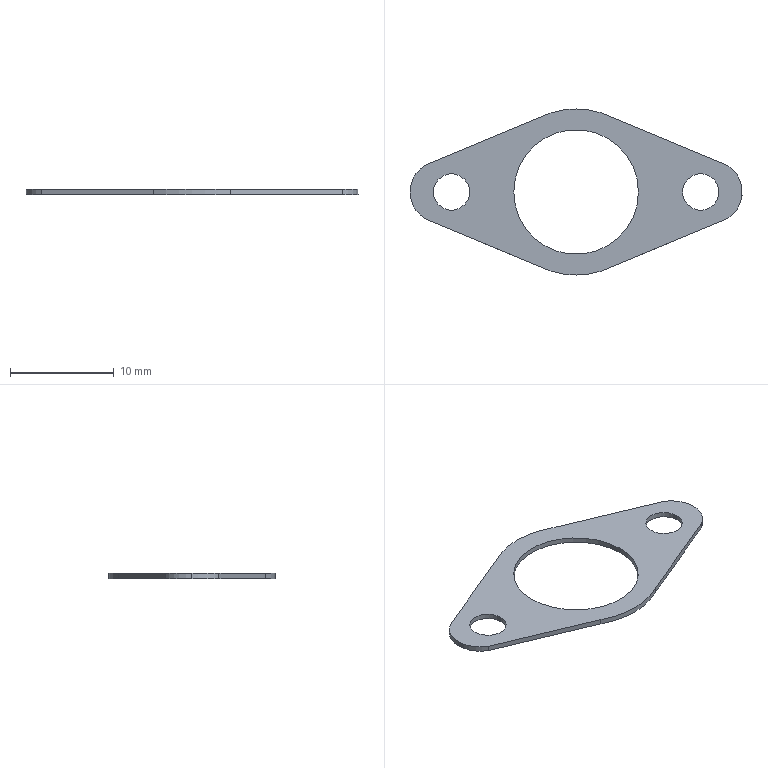Part | STEP file | WENKONG2_1_1_1_1 | 1 solid | 17 faces | box 32 x 16 x 0.5 mm | volume 101.047 mm3 | cylinder 11 | plane 6 | commonest cylinder face diameters 3.5 x4 6 x3 12 x2 16 x2
STEP:
#1=CARTESIAN_POINT('',(0.,0.,0.));
#2=DIRECTION('',(0.,0.,1.));
#3=DIRECTION('',(1.,0.,0.));
#4=AXIS2_PLACEMENT_3D('',#1,#2,#3);
#5=CARTESIAN_POINT('',(10.25,0.,0.));
#6=VERTEX_POINT('',#5);
#7=CARTESIAN_POINT('',(10.25,0.,0.5));
#8=VERTEX_POINT('',#7);
#9=CARTESIAN_POINT('',(10.25,0.,0.));
#10=DIRECTION('',(0.,0.,1.));
#11=VECTOR('',#10,0.5);
#12=LINE('',#9,#11);
#13=EDGE_CURVE('',#6,#8,#12,.T.);
#14=ORIENTED_EDGE('',*,*,#13,.F.);
#15=CARTESIAN_POINT('',(13.75,0.,0.));
#16=VERTEX_POINT('',#15);
#17=CARTESIAN_POINT('',(12.,0.,0.));
#18=DIRECTION('',(0.,0.,-1.));
#19=DIRECTION('',(1.,0.,0.));
#20=AXIS2_PLACEMENT_3D('',#17,#18,#19);
#21=CIRCLE('',#20,1.75);
#22=EDGE_CURVE('',#16,#6,#21,.T.);
#23=ORIENTED_EDGE('',*,*,#22,.F.);
#24=CARTESIAN_POINT('',(13.75,0.,0.5));
#25=VERTEX_POINT('',#24);
#26=CARTESIAN_POINT('',(13.75,0.,0.5));
#27=DIRECTION('',(0.,0.,-1.));
#28=VECTOR('',#27,0.5);
#29=LINE('',#26,#28);
#30=EDGE_CURVE('',#25,#16,#29,.T.);
#31=ORIENTED_EDGE('',*,*,#30,.F.);
#32=CARTESIAN_POINT('',(12.,0.,0.5));
#33=DIRECTION('',(0.,0.,1.));
#34=DIRECTION('',(-1.,0.,0.));
#35=AXIS2_PLACEMENT_3D('',#32,#33,#34);
#36=CIRCLE('',#35,1.75);
#37=EDGE_CURVE('',#8,#25,#36,.T.);
#38=ORIENTED_EDGE('',*,*,#37,.F.);
#39=EDGE_LOOP('',(#14,#23,#31,#38));
#40=FACE_OUTER_BOUND('',#39,.F.);
#41=CARTESIAN_POINT('',(12.,0.,0.25));
#42=DIRECTION('',(0.,0.,-1.));
#43=DIRECTION('',(1.,0.,0.));
#44=AXIS2_PLACEMENT_3D('',#41,#42,#43);
#45=CYLINDRICAL_SURFACE('',#44,1.75);
#46=ADVANCED_FACE('',(#40),#45,.F.);
#47=CARTESIAN_POINT('',(12.,0.,0.));
#48=DIRECTION('',(0.,0.,-1.));
#49=DIRECTION('',(-1.,0.,0.));
#50=AXIS2_PLACEMENT_3D('',#47,#48,#49);
#51=CIRCLE('',#50,1.75);
#52=EDGE_CURVE('',#6,#16,#51,.T.);
#53=ORIENTED_EDGE('',*,*,#52,.F.);
#54=ORIENTED_EDGE('',*,*,#13,.T.);
#55=CARTESIAN_POINT('',(12.,0.,0.5));
#56=DIRECTION('',(0.,0.,1.));
#57=DIRECTION('',(1.,0.,0.));
#58=AXIS2_PLACEMENT_3D('',#55,#56,#57);
#59=CIRCLE('',#58,1.75);
#60=EDGE_CURVE('',#25,#8,#59,.T.);
#61=ORIENTED_EDGE('',*,*,#60,.F.);
#62=ORIENTED_EDGE('',*,*,#30,.T.);
#63=EDGE_LOOP('',(#53,#54,#61,#62));
#64=FACE_OUTER_BOUND('',#63,.F.);
#65=CARTESIAN_POINT('',(12.,0.,0.25));
#66=DIRECTION('',(0.,0.,-1.));
#67=DIRECTION('',(-1.,0.,0.));
#68=AXIS2_PLACEMENT_3D('',#65,#66,#67);
#69=CYLINDRICAL_SURFACE('',#68,1.75);
#70=ADVANCED_FACE('',(#64),#69,.F.);
#71=CARTESIAN_POINT('',(-16.,0.000000002,0.));
#72=VERTEX_POINT('',#71);
#73=CARTESIAN_POINT('',(-14.499,-2.599,0.));
#74=VERTEX_POINT('',#73);
#75=CARTESIAN_POINT('',(-13.,0.,0.));
#76=DIRECTION('',(0.,0.,1.));
#77=DIRECTION('',(-1.,0.000000001,0.));
#78=AXIS2_PLACEMENT_3D('',#75,#76,#77);
#79=CIRCLE('',#78,3.);
#80=EDGE_CURVE('',#72,#74,#79,.T.);
#81=ORIENTED_EDGE('',*,*,#80,.T.);
#82=CARTESIAN_POINT('',(-3.692,-7.097,0.));
#83=VERTEX_POINT('',#82);
#84=CARTESIAN_POINT('',(-14.499,-2.599,0.));
#85=DIRECTION('',(0.9232,-0.3843,0.));
#86=VECTOR('',#85,11.706);
#87=LINE('',#84,#86);
#88=EDGE_CURVE('',#74,#83,#87,.T.);
#89=ORIENTED_EDGE('',*,*,#88,.T.);
#90=CARTESIAN_POINT('',(3.692,-7.097,0.));
#91=VERTEX_POINT('',#90);
#92=CARTESIAN_POINT('',(0.,-0.000000001,0.));
#93=DIRECTION('',(0.,0.,1.));
#94=DIRECTION('',(-0.4615,-0.8871,0.));
#95=AXIS2_PLACEMENT_3D('',#92,#93,#94);
#96=CIRCLE('',#95,8.);
#97=EDGE_CURVE('',#83,#91,#96,.T.);
#98=ORIENTED_EDGE('',*,*,#97,.T.);
#99=CARTESIAN_POINT('',(14.499,-2.599,0.));
#100=VERTEX_POINT('',#99);
#101=CARTESIAN_POINT('',(3.692,-7.097,0.));
#102=DIRECTION('',(0.9232,0.3843,0.));
#103=VECTOR('',#102,11.706);
#104=LINE('',#101,#103);
#105=EDGE_CURVE('',#91,#100,#104,.T.);
#106=ORIENTED_EDGE('',*,*,#105,.T.);
#107=CARTESIAN_POINT('',(14.499,2.599,0.));
#108=VERTEX_POINT('',#107);
#109=CARTESIAN_POINT('',(13.,0.,0.));
#110=DIRECTION('',(0.,0.,1.));
#111=DIRECTION('',(0.4997,-0.8662,0.));
#112=AXIS2_PLACEMENT_3D('',#109,#110,#111);
#113=CIRCLE('',#112,3.);
#114=EDGE_CURVE('',#100,#108,#113,.T.);
#115=ORIENTED_EDGE('',*,*,#114,.T.);
#116=CARTESIAN_POINT('',(3.692,7.097,0.));
#117=VERTEX_POINT('',#116);
#118=CARTESIAN_POINT('',(14.499,2.599,0.));
#119=DIRECTION('',(-0.9232,0.3843,0.));
#120=VECTOR('',#119,11.706);
#121=LINE('',#118,#120);
#122=EDGE_CURVE('',#108,#117,#121,.T.);
#123=ORIENTED_EDGE('',*,*,#122,.T.);
#124=CARTESIAN_POINT('',(-3.692,7.097,0.));
#125=VERTEX_POINT('',#124);
#126=CARTESIAN_POINT('',(0.,0.000000001,0.));
#127=DIRECTION('',(0.,0.,1.));
#128=DIRECTION('',(0.4615,0.8871,0.));
#129=AXIS2_PLACEMENT_3D('',#126,#127,#128);
#130=CIRCLE('',#129,8.);
#131=EDGE_CURVE('',#117,#125,#130,.T.);
#132=ORIENTED_EDGE('',*,*,#131,.T.);
#133=CARTESIAN_POINT('',(-14.499,2.599,0.));
#134=VERTEX_POINT('',#133);
#135=CARTESIAN_POINT('',(-3.692,7.097,0.));
#136=DIRECTION('',(-0.9232,-0.3843,0.));
#137=VECTOR('',#136,11.706);
#138=LINE('',#135,#137);
#139=EDGE_CURVE('',#125,#134,#138,.T.);
#140=ORIENTED_EDGE('',*,*,#139,.T.);
#141=CARTESIAN_POINT('',(-13.,0.,0.));
#142=DIRECTION('',(0.,0.,1.));
#143=DIRECTION('',(-0.4997,0.8662,0.));
#144=AXIS2_PLACEMENT_3D('',#141,#142,#143);
#145=CIRCLE('',#144,3.);
#146=EDGE_CURVE('',#134,#72,#145,.T.);
#147=ORIENTED_EDGE('',*,*,#146,.T.);
#148=EDGE_LOOP('',(#81,#89,#98,#106,#115,#123,#132,#140,#147));
#149=FACE_OUTER_BOUND('',#148,.F.);
#150=CARTESIAN_POINT('',(-6.,0.,0.));
#151=VERTEX_POINT('',#150);
#152=CARTESIAN_POINT('',(6.,0.,0.));
#153=VERTEX_POINT('',#152);
#154=CARTESIAN_POINT('',(0.,0.,0.));
#155=DIRECTION('',(0.,0.,-1.));
#156=DIRECTION('',(-1.,0.,0.));
#157=AXIS2_PLACEMENT_3D('',#154,#155,#156);
#158=CIRCLE('',#157,6.);
#159=EDGE_CURVE('',#151,#153,#158,.T.);
#160=ORIENTED_EDGE('',*,*,#159,.T.);
#161=CARTESIAN_POINT('',(0.,0.,0.));
#162=DIRECTION('',(0.,0.,-1.));
#163=DIRECTION('',(1.,0.,0.));
#164=AXIS2_PLACEMENT_3D('',#161,#162,#163);
#165=CIRCLE('',#164,6.);
#166=EDGE_CURVE('',#153,#151,#165,.T.);
#167=ORIENTED_EDGE('',*,*,#166,.T.);
#168=EDGE_LOOP('',(#160,#167));
#169=FACE_BOUND('',#168,.F.);
#170=CARTESIAN_POINT('',(-13.75,0.,0.));
#171=VERTEX_POINT('',#170);
#172=CARTESIAN_POINT('',(-10.25,0.,0.));
#173=VERTEX_POINT('',#172);
#174=CARTESIAN_POINT('',(-12.,0.,0.));
#175=DIRECTION('',(0.,0.,-1.));
#176=DIRECTION('',(-1.,0.,0.));
#177=AXIS2_PLACEMENT_3D('',#174,#175,#176);
#178=CIRCLE('',#177,1.75);
#179=EDGE_CURVE('',#171,#173,#178,.T.);
#180=ORIENTED_EDGE('',*,*,#179,.T.);
#181=CARTESIAN_POINT('',(-12.,0.,0.));
#182=DIRECTION('',(0.,0.,-1.));
#183=DIRECTION('',(1.,0.,0.));
#184=AXIS2_PLACEMENT_3D('',#181,#182,#183);
#185=CIRCLE('',#184,1.75);
#186=EDGE_CURVE('',#173,#171,#185,.T.);
#187=ORIENTED_EDGE('',*,*,#186,.T.);
#188=EDGE_LOOP('',(#180,#187));
#189=FACE_BOUND('',#188,.F.);
#190=ORIENTED_EDGE('',*,*,#52,.T.);
#191=ORIENTED_EDGE('',*,*,#22,.T.);
#192=EDGE_LOOP('',(#190,#191));
#193=FACE_BOUND('',#192,.F.);
#194=CARTESIAN_POINT('',(0.001966,0.,0.));
#195=DIRECTION('',(0.,0.,1.));
#196=DIRECTION('',(1.,0.,0.));
#197=AXIS2_PLACEMENT_3D('',#194,#195,#196);
#198=PLANE('',#197);
#199=ADVANCED_FACE('',(#149,#169,#189,#193),#198,.F.);
#200=CARTESIAN_POINT('',(-14.499,-2.599,0.5));
#201=VERTEX_POINT('',#200);
#202=CARTESIAN_POINT('',(-16.,0.000000002,0.5));
#203=VERTEX_POINT('',#202);
#204=CARTESIAN_POINT('',(-13.,0.,0.5));
#205=DIRECTION('',(0.,0.,-1.));
#206=DIRECTION('',(-0.4997,-0.8662,0.));
#207=AXIS2_PLACEMENT_3D('',#204,#205,#206);
#208=CIRCLE('',#207,3.);
#209=EDGE_CURVE('',#201,#203,#208,.T.);
#210=ORIENTED_EDGE('',*,*,#209,.F.);
#211=CARTESIAN_POINT('',(-14.499,-2.599,0.5));
#212=DIRECTION('',(0.,0.,-1.));
#213=VECTOR('',#212,0.5);
#214=LINE('',#211,#213);
#215=EDGE_CURVE('',#201,#74,#214,.T.);
#216=ORIENTED_EDGE('',*,*,#215,.T.);
#217=ORIENTED_EDGE('',*,*,#80,.F.);
#218=CARTESIAN_POINT('',(-16.,0.000000001,0.));
#219=DIRECTION('',(0.,0.,1.));
#220=VECTOR('',#219,0.5);
#221=LINE('',#218,#220);
#222=EDGE_CURVE('',#72,#203,#221,.T.);
#223=ORIENTED_EDGE('',*,*,#222,.T.);
#224=EDGE_LOOP('',(#210,#216,#217,#223));
#225=FACE_OUTER_BOUND('',#224,.F.);
#226=CARTESIAN_POINT('',(-13.,0.,0.25));
#227=DIRECTION('',(0.,0.,-1.));
#228=DIRECTION('',(-0.4997,-0.8662,0.));
#229=AXIS2_PLACEMENT_3D('',#226,#227,#228);
#230=CYLINDRICAL_SURFACE('',#229,3.);
#231=ADVANCED_FACE('',(#225),#230,.T.);
#232=CARTESIAN_POINT('',(-14.499,2.599,0.5));
#233=VERTEX_POINT('',#232);
#234=CARTESIAN_POINT('',(-13.,0.,0.5));
#235=DIRECTION('',(0.,0.,-1.));
#236=DIRECTION('',(-1.,0.000000001,0.));
#237=AXIS2_PLACEMENT_3D('',#234,#235,#236);
#238=CIRCLE('',#237,3.);
#239=EDGE_CURVE('',#203,#233,#238,.T.);
#240=ORIENTED_EDGE('',*,*,#239,.T.);
#241=CARTESIAN_POINT('',(-3.692,7.097,0.5));
#242=VERTEX_POINT('',#241);
#243=CARTESIAN_POINT('',(-14.499,2.599,0.5));
#244=DIRECTION('',(0.9232,0.3843,0.));
#245=VECTOR('',#244,11.706);
#246=LINE('',#243,#245);
#247=EDGE_CURVE('',#233,#242,#246,.T.);
#248=ORIENTED_EDGE('',*,*,#247,.T.);
#249=CARTESIAN_POINT('',(3.692,7.097,0.5));
#250=VERTEX_POINT('',#249);
#251=CARTESIAN_POINT('',(0.,0.000000001,0.5));
#252=DIRECTION('',(0.,0.,-1.));
#253=DIRECTION('',(-0.4615,0.8871,0.));
#254=AXIS2_PLACEMENT_3D('',#251,#252,#253);
#255=CIRCLE('',#254,8.);
#256=EDGE_CURVE('',#242,#250,#255,.T.);
#257=ORIENTED_EDGE('',*,*,#256,.T.);
#258=CARTESIAN_POINT('',(14.499,2.599,0.5));
#259=VERTEX_POINT('',#258);
#260=CARTESIAN_POINT('',(3.692,7.097,0.5));
#261=DIRECTION('',(0.9232,-0.3843,0.));
#262=VECTOR('',#261,11.706);
#263=LINE('',#260,#262);
#264=EDGE_CURVE('',#250,#259,#263,.T.);
#265=ORIENTED_EDGE('',*,*,#264,.T.);
#266=CARTESIAN_POINT('',(14.499,-2.599,0.5));
#267=VERTEX_POINT('',#266);
#268=CARTESIAN_POINT('',(13.,0.,0.5));
#269=DIRECTION('',(0.,0.,-1.));
#270=DIRECTION('',(0.4997,0.8662,0.));
#271=AXIS2_PLACEMENT_3D('',#268,#269,#270);
#272=CIRCLE('',#271,3.);
#273=EDGE_CURVE('',#259,#267,#272,.T.);
#274=ORIENTED_EDGE('',*,*,#273,.T.);
#275=CARTESIAN_POINT('',(3.692,-7.097,0.5));
#276=VERTEX_POINT('',#275);
#277=CARTESIAN_POINT('',(14.499,-2.599,0.5));
#278=DIRECTION('',(-0.9232,-0.3843,0.));
#279=VECTOR('',#278,11.706);
#280=LINE('',#277,#279);
#281=EDGE_CURVE('',#267,#276,#280,.T.);
#282=ORIENTED_EDGE('',*,*,#281,.T.);
#283=CARTESIAN_POINT('',(-3.692,-7.097,0.5));
#284=VERTEX_POINT('',#283);
#285=CARTESIAN_POINT('',(0.,-0.000000001,0.5));
#286=DIRECTION('',(0.,0.,-1.));
#287=DIRECTION('',(0.4615,-0.8871,0.));
#288=AXIS2_PLACEMENT_3D('',#285,#286,#287);
#289=CIRCLE('',#288,8.);
#290=EDGE_CURVE('',#276,#284,#289,.T.);
#291=ORIENTED_EDGE('',*,*,#290,.T.);
#292=CARTESIAN_POINT('',(-3.692,-7.097,0.5));
#293=DIRECTION('',(-0.9232,0.3843,0.));
#294=VECTOR('',#293,11.706);
#295=LINE('',#292,#294);
#296=EDGE_CURVE('',#284,#201,#295,.T.);
#297=ORIENTED_EDGE('',*,*,#296,.T.);
#298=ORIENTED_EDGE('',*,*,#209,.T.);
#299=EDGE_LOOP('',(#240,#248,#257,#265,#274,#282,#291,#297,#298));
#300=FACE_OUTER_BOUND('',#299,.F.);
#301=CARTESIAN_POINT('',(-13.75,0.,0.5));
#302=VERTEX_POINT('',#301);
#303=CARTESIAN_POINT('',(-10.25,0.,0.5));
#304=VERTEX_POINT('',#303);
#305=CARTESIAN_POINT('',(-12.,0.,0.5));
#306=DIRECTION('',(0.,0.,1.));
#307=DIRECTION('',(-1.,0.,0.));
#308=AXIS2_PLACEMENT_3D('',#305,#306,#307);
#309=CIRCLE('',#308,1.75);
#310=EDGE_CURVE('',#302,#304,#309,.T.);
#311=ORIENTED_EDGE('',*,*,#310,.T.);
#312=CARTESIAN_POINT('',(-12.,0.,0.5));
#313=DIRECTION('',(0.,0.,1.));
#314=DIRECTION('',(1.,0.,0.));
#315=AXIS2_PLACEMENT_3D('',#312,#313,#314);
#316=CIRCLE('',#315,1.75);
#317=EDGE_CURVE('',#304,#302,#316,.T.);
#318=ORIENTED_EDGE('',*,*,#317,.T.);
#319=EDGE_LOOP('',(#311,#318));
#320=FACE_BOUND('',#319,.F.);
#321=CARTESIAN_POINT('',(-6.,0.,0.5));
#322=VERTEX_POINT('',#321);
#323=CARTESIAN_POINT('',(6.,0.,0.5));
#324=VERTEX_POINT('',#323);
#325=CARTESIAN_POINT('',(0.,0.,0.5));
#326=DIRECTION('',(0.,0.,1.));
#327=DIRECTION('',(-1.,0.,0.));
#328=AXIS2_PLACEMENT_3D('',#325,#326,#327);
#329=CIRCLE('',#328,6.);
#330=EDGE_CURVE('',#322,#324,#329,.T.);
#331=ORIENTED_EDGE('',*,*,#330,.T.);
#332=CARTESIAN_POINT('',(0.,0.,0.5));
#333=DIRECTION('',(0.,0.,1.));
#334=DIRECTION('',(1.,0.,0.));
#335=AXIS2_PLACEMENT_3D('',#332,#333,#334);
#336=CIRCLE('',#335,6.);
#337=EDGE_CURVE('',#324,#322,#336,.T.);
#338=ORIENTED_EDGE('',*,*,#337,.T.);
#339=EDGE_LOOP('',(#331,#338));
#340=FACE_BOUND('',#339,.F.);
#341=ORIENTED_EDGE('',*,*,#37,.T.);
#342=ORIENTED_EDGE('',*,*,#60,.T.);
#343=EDGE_LOOP('',(#341,#342));
#344=FACE_BOUND('',#343,.F.);
#345=CARTESIAN_POINT('',(0.001966,0.,0.5));
#346=DIRECTION('',(0.,0.,1.));
#347=DIRECTION('',(1.,0.,0.));
#348=AXIS2_PLACEMENT_3D('',#345,#346,#347);
#349=PLANE('',#348);
#350=ADVANCED_FACE('',(#300,#320,#340,#344),#349,.T.);
#351=ORIENTED_EDGE('',*,*,#222,.F.);
#352=ORIENTED_EDGE('',*,*,#146,.F.);
#353=CARTESIAN_POINT('',(-14.499,2.599,0.));
#354=DIRECTION('',(0.,0.,1.));
#355=VECTOR('',#354,0.5);
#356=LINE('',#353,#355);
#357=EDGE_CURVE('',#134,#233,#356,.T.);
#358=ORIENTED_EDGE('',*,*,#357,.T.);
#359=ORIENTED_EDGE('',*,*,#239,.F.);
#360=EDGE_LOOP('',(#351,#352,#358,#359));
#361=FACE_OUTER_BOUND('',#360,.F.);
#362=CARTESIAN_POINT('',(-13.,0.,0.25));
#363=DIRECTION('',(0.,0.,-1.));
#364=DIRECTION('',(-1.,0.,0.));
#365=AXIS2_PLACEMENT_3D('',#362,#363,#364);
#366=CYLINDRICAL_SURFACE('',#365,3.);
#367=ADVANCED_FACE('',(#361),#366,.T.);
#368=CARTESIAN_POINT('',(-3.692,7.097,0.5));
#369=DIRECTION('',(0.000000001,0.000000001,-1.));
#370=VECTOR('',#369,0.5);
#371=LINE('',#368,#370);
#372=EDGE_CURVE('',#242,#125,#371,.T.);
#373=ORIENTED_EDGE('',*,*,#372,.F.);
#374=ORIENTED_EDGE('',*,*,#247,.F.);
#375=ORIENTED_EDGE('',*,*,#357,.F.);
#376=ORIENTED_EDGE('',*,*,#139,.F.);
#377=EDGE_LOOP('',(#373,#374,#375,#376));
#378=FACE_OUTER_BOUND('',#377,.F.);
#379=CARTESIAN_POINT('',(-9.096,4.848,0.25));
#380=DIRECTION('',(-0.3843,0.9232,0.));
#381=DIRECTION('',(0.9232,0.3843,0.));
#382=AXIS2_PLACEMENT_3D('',#379,#380,#381);
#383=PLANE('',#382);
#384=ADVANCED_FACE('',(#378),#383,.T.);
#385=ORIENTED_EDGE('',*,*,#131,.F.);
#386=CARTESIAN_POINT('',(3.692,7.097,0.));
#387=DIRECTION('',(0.,0.,1.));
#388=VECTOR('',#387,0.5);
#389=LINE('',#386,#388);
#390=EDGE_CURVE('',#117,#250,#389,.T.);
#391=ORIENTED_EDGE('',*,*,#390,.T.);
#392=ORIENTED_EDGE('',*,*,#256,.F.);
#393=ORIENTED_EDGE('',*,*,#372,.T.);
#394=EDGE_LOOP('',(#385,#391,#392,#393));
#395=FACE_OUTER_BOUND('',#394,.F.);
#396=CARTESIAN_POINT('',(0.,0.000000001,0.25));
#397=DIRECTION('',(0.,0.,-1.));
#398=DIRECTION('',(-0.4615,0.8871,0.));
#399=AXIS2_PLACEMENT_3D('',#396,#397,#398);
#400=CYLINDRICAL_SURFACE('',#399,8.);
#401=ADVANCED_FACE('',(#395),#400,.T.);
#402=CARTESIAN_POINT('',(14.499,2.599,0.5));
#403=DIRECTION('',(0.,0.,-1.));
#404=VECTOR('',#403,0.5);
#405=LINE('',#402,#404);
#406=EDGE_CURVE('',#259,#108,#405,.T.);
#407=ORIENTED_EDGE('',*,*,#406,.F.);
#408=ORIENTED_EDGE('',*,*,#264,.F.);
#409=ORIENTED_EDGE('',*,*,#390,.F.);
#410=ORIENTED_EDGE('',*,*,#122,.F.);
#411=EDGE_LOOP('',(#407,#408,#409,#410));
#412=FACE_OUTER_BOUND('',#411,.F.);
#413=CARTESIAN_POINT('',(9.096,4.848,0.25));
#414=DIRECTION('',(0.3843,0.9232,0.));
#415=DIRECTION('',(0.9232,-0.3843,0.));
#416=AXIS2_PLACEMENT_3D('',#413,#414,#415);
#417=PLANE('',#416);
#418=ADVANCED_FACE('',(#412),#417,.T.);
#419=ORIENTED_EDGE('',*,*,#114,.F.);
#420=CARTESIAN_POINT('',(14.499,-2.599,0.));
#421=DIRECTION('',(0.,0.,1.));
#422=VECTOR('',#421,0.5);
#423=LINE('',#420,#422);
#424=EDGE_CURVE('',#100,#267,#423,.T.);
#425=ORIENTED_EDGE('',*,*,#424,.T.);
#426=ORIENTED_EDGE('',*,*,#273,.F.);
#427=ORIENTED_EDGE('',*,*,#406,.T.);
#428=EDGE_LOOP('',(#419,#425,#426,#427));
#429=FACE_OUTER_BOUND('',#428,.F.);
#430=CARTESIAN_POINT('',(13.,0.,0.25));
#431=DIRECTION('',(0.,0.,-1.));
#432=DIRECTION('',(0.4997,0.8662,0.));
#433=AXIS2_PLACEMENT_3D('',#430,#431,#432);
#434=CYLINDRICAL_SURFACE('',#433,3.);
#435=ADVANCED_FACE('',(#429),#434,.T.);
#436=CARTESIAN_POINT('',(3.692,-7.097,0.5));
#437=DIRECTION('',(0.000000001,0.,-1.));
#438=VECTOR('',#437,0.5);
#439=LINE('',#436,#438);
#440=EDGE_CURVE('',#276,#91,#439,.T.);
#441=ORIENTED_EDGE('',*,*,#440,.F.);
#442=ORIENTED_EDGE('',*,*,#281,.F.);
#443=ORIENTED_EDGE('',*,*,#424,.F.);
#444=ORIENTED_EDGE('',*,*,#105,.F.);
#445=EDGE_LOOP('',(#441,#442,#443,#444));
#446=FACE_OUTER_BOUND('',#445,.F.);
#447=CARTESIAN_POINT('',(9.096,-4.848,0.25));
#448=DIRECTION('',(-0.3843,0.9232,0.));
#449=DIRECTION('',(-0.9232,-0.3843,0.));
#450=AXIS2_PLACEMENT_3D('',#447,#448,#449);
#451=PLANE('',#450);
#452=ADVANCED_FACE('',(#446),#451,.F.);
#453=ORIENTED_EDGE('',*,*,#97,.F.);
#454=CARTESIAN_POINT('',(-3.692,-7.097,0.));
#455=DIRECTION('',(0.000000001,0.,1.));
#456=VECTOR('',#455,0.5);
#457=LINE('',#454,#456);
#458=EDGE_CURVE('',#83,#284,#457,.T.);
#459=ORIENTED_EDGE('',*,*,#458,.T.);
#460=ORIENTED_EDGE('',*,*,#290,.F.);
#461=ORIENTED_EDGE('',*,*,#440,.T.);
#462=EDGE_LOOP('',(#453,#459,#460,#461));
#463=FACE_OUTER_BOUND('',#462,.F.);
#464=CARTESIAN_POINT('',(0.,-0.000000001,0.25));
#465=DIRECTION('',(0.,0.,-1.));
#466=DIRECTION('',(0.4615,-0.8871,0.));
#467=AXIS2_PLACEMENT_3D('',#464,#465,#466);
#468=CYLINDRICAL_SURFACE('',#467,8.);
#469=ADVANCED_FACE('',(#463),#468,.T.);
#470=ORIENTED_EDGE('',*,*,#215,.F.);
#471=ORIENTED_EDGE('',*,*,#296,.F.);
#472=ORIENTED_EDGE('',*,*,#458,.F.);
#473=ORIENTED_EDGE('',*,*,#88,.F.);
#474=EDGE_LOOP('',(#470,#471,#472,#473));
#475=FACE_OUTER_BOUND('',#474,.F.);
#476=CARTESIAN_POINT('',(-9.096,-4.848,0.25));
#477=DIRECTION('',(0.3843,0.9232,0.));
#478=DIRECTION('',(-0.9232,0.3843,0.));
#479=AXIS2_PLACEMENT_3D('',#476,#477,#478);
#480=PLANE('',#479);
#481=ADVANCED_FACE('',(#475),#480,.F.);
#482=CARTESIAN_POINT('',(-13.75,0.,0.));
#483=DIRECTION('',(0.,0.,1.));
#484=VECTOR('',#483,0.5);
#485=LINE('',#482,#484);
#486=EDGE_CURVE('',#171,#302,#485,.T.);
#487=ORIENTED_EDGE('',*,*,#486,.F.);
#488=ORIENTED_EDGE('',*,*,#186,.F.);
#489=CARTESIAN_POINT('',(-10.25,0.,0.5));
#490=DIRECTION('',(0.,0.,-1.));
#491=VECTOR('',#490,0.5);
#492=LINE('',#489,#491);
#493=EDGE_CURVE('',#304,#173,#492,.T.);
#494=ORIENTED_EDGE('',*,*,#493,.F.);
#495=ORIENTED_EDGE('',*,*,#310,.F.);
#496=EDGE_LOOP('',(#487,#488,#494,#495));
#497=FACE_OUTER_BOUND('',#496,.F.);
#498=CARTESIAN_POINT('',(-12.,0.,0.25));
#499=DIRECTION('',(0.,0.,-1.));
#500=DIRECTION('',(1.,0.,0.));
#501=AXIS2_PLACEMENT_3D('',#498,#499,#500);
#502=CYLINDRICAL_SURFACE('',#501,1.75);
#503=ADVANCED_FACE('',(#497),#502,.F.);
#504=ORIENTED_EDGE('',*,*,#179,.F.);
#505=ORIENTED_EDGE('',*,*,#486,.T.);
#506=ORIENTED_EDGE('',*,*,#317,.F.);
#507=ORIENTED_EDGE('',*,*,#493,.T.);
#508=EDGE_LOOP('',(#504,#505,#506,#507));
#509=FACE_OUTER_BOUND('',#508,.F.);
#510=CARTESIAN_POINT('',(-12.,0.,0.25));
#511=DIRECTION('',(0.,0.,-1.));
#512=DIRECTION('',(-1.,0.,0.));
#513=AXIS2_PLACEMENT_3D('',#510,#511,#512);
#514=CYLINDRICAL_SURFACE('',#513,1.75);
#515=ADVANCED_FACE('',(#509),#514,.F.);
#516=CARTESIAN_POINT('',(-6.,0.,0.));
#517=DIRECTION('',(0.,0.,1.));
#518=VECTOR('',#517,0.5);
#519=LINE('',#516,#518);
#520=EDGE_CURVE('',#151,#322,#519,.T.);
#521=ORIENTED_EDGE('',*,*,#520,.F.);
#522=ORIENTED_EDGE('',*,*,#166,.F.);
#523=CARTESIAN_POINT('',(6.,0.,0.5));
#524=DIRECTION('',(0.,0.,-1.));
#525=VECTOR('',#524,0.5);
#526=LINE('',#523,#525);
#527=EDGE_CURVE('',#324,#153,#526,.T.);
#528=ORIENTED_EDGE('',*,*,#527,.F.);
#529=ORIENTED_EDGE('',*,*,#330,.F.);
#530=EDGE_LOOP('',(#521,#522,#528,#529));
#531=FACE_OUTER_BOUND('',#530,.F.);
#532=CARTESIAN_POINT('',(0.,0.,0.25));
#533=DIRECTION('',(0.,0.,-1.));
#534=DIRECTION('',(1.,0.,0.));
#535=AXIS2_PLACEMENT_3D('',#532,#533,#534);
#536=CYLINDRICAL_SURFACE('',#535,6.);
#537=ADVANCED_FACE('',(#531),#536,.F.);
#538=ORIENTED_EDGE('',*,*,#159,.F.);
#539=ORIENTED_EDGE('',*,*,#520,.T.);
#540=ORIENTED_EDGE('',*,*,#337,.F.);
#541=ORIENTED_EDGE('',*,*,#527,.T.);
#542=EDGE_LOOP('',(#538,#539,#540,#541));
#543=FACE_OUTER_BOUND('',#542,.F.);
#544=CARTESIAN_POINT('',(0.,0.,0.25));
#545=DIRECTION('',(0.,0.,-1.));
#546=DIRECTION('',(-1.,0.,0.));
#547=AXIS2_PLACEMENT_3D('',#544,#545,#546);
#548=CYLINDRICAL_SURFACE('',#547,6.);
#549=ADVANCED_FACE('',(#543),#548,.F.);
#550=CLOSED_SHELL('',(#46,#70,#199,#231,#350,#367,#384,#401,#418,#435,#452,#469,#481,#503,#515,#537,#549));
#551=MANIFOLD_SOLID_BREP('',#550);
#552=(LENGTH_UNIT()NAMED_UNIT(*)SI_UNIT(.MILLI.,.METRE.));
#553=UNCERTAINTY_MEASURE_WITH_UNIT(LENGTH_MEASURE(0.003579),#552,'','');
#554=(NAMED_UNIT(*)PLANE_ANGLE_UNIT()SI_UNIT($,.RADIAN.));
#555=PLANE_ANGLE_MEASURE_WITH_UNIT(PLANE_ANGLE_MEASURE(0.01745),#554);
#556=(CONVERSION_BASED_UNIT('DEGREE',#555)NAMED_UNIT(*)PLANE_ANGLE_UNIT());
#557=(NAMED_UNIT(*)SI_UNIT($,.STERADIAN.)SOLID_ANGLE_UNIT());
#558=(GEOMETRIC_REPRESENTATION_CONTEXT(3)GLOBAL_UNCERTAINTY_ASSIGNED_CONTEXT((#553))GLOBAL_UNIT_ASSIGNED_CONTEXT((#552,#556,#557))REPRESENTATION_CONTEXT('',''));
#559=ADVANCED_BREP_SHAPE_REPRESENTATION('',(#4,#551),#558);